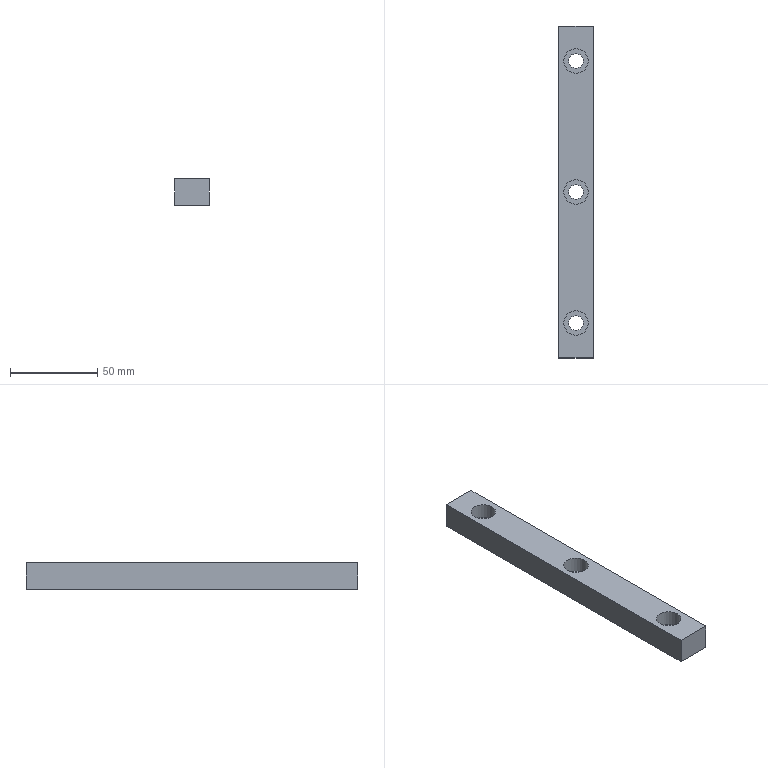Part | STEP file | YBQDJ-QD-4 | 1 solid | 15 faces | box 20 x 190 x 15 mm | volume 51822 mm3 | plane 9 | cylinder 6 | commonest cylinder face diameters 8.5 x3 14 x3
STEP:
#1=CARTESIAN_POINT('',(0.,0.,0.));
#2=DIRECTION('',(0.,0.,1.));
#3=DIRECTION('',(1.,0.,0.));
#4=AXIS2_PLACEMENT_3D('',#1,#2,#3);
#5=CARTESIAN_POINT('',(-330.,-100.,120.));
#6=VERTEX_POINT('',#5);
#7=CARTESIAN_POINT('',(-330.,-290.,120.));
#8=VERTEX_POINT('',#7);
#9=CARTESIAN_POINT('',(-330.,-85.,120.));
#10=DIRECTION('',(0.,-1.,0.));
#11=VECTOR('',#10,1.);
#12=LINE('',#9,#11);
#13=CARTESIAN_POINT('',(-330.,-85.,135.));
#14=DIRECTION('',(1.,0.,0.));
#15=DIRECTION('',(0.,0.,-1.));
#16=AXIS2_PLACEMENT_3D('',#13,#14,#15);
#17=PLANE('',#16);
#18=CARTESIAN_POINT('',(15.,0.));
#19=DIRECTION('',(0.,-1.));
#20=VECTOR('',#19,1.);
#21=LINE('',#18,#20);
#22=(GEOMETRIC_REPRESENTATION_CONTEXT(2)PARAMETRIC_REPRESENTATION_CONTEXT()REPRESENTATION_CONTEXT('',''));
#23=DEFINITIONAL_REPRESENTATION('',(#21),#22);
#24=PCURVE('',#17,#23);
#25=CARTESIAN_POINT('',(92.5,0.000000001,120.));
#26=DIRECTION('',(0.,0.,1.));
#27=DIRECTION('',(1.,0.,0.));
#28=AXIS2_PLACEMENT_3D('',#25,#26,#27);
#29=PLANE('',#28);
#30=CARTESIAN_POINT('',(-422.5,-85.));
#31=DIRECTION('',(0.,-1.));
#32=VECTOR('',#31,1.);
#33=LINE('',#30,#32);
#34=(GEOMETRIC_REPRESENTATION_CONTEXT(2)PARAMETRIC_REPRESENTATION_CONTEXT()REPRESENTATION_CONTEXT('',''));
#35=DEFINITIONAL_REPRESENTATION('',(#33),#34);
#36=PCURVE('',#29,#35);
#37=SURFACE_CURVE('',#12,(#24,#36),.PCURVE_S1.);
#38=EDGE_CURVE('',#6,#8,#37,.T.);
#39=ORIENTED_EDGE('',*,*,#38,.T.);
#40=CARTESIAN_POINT('',(-330.,-290.,135.));
#41=VERTEX_POINT('',#40);
#42=CARTESIAN_POINT('',(-330.,-290.,9.));
#43=DIRECTION('',(0.,0.,-1.));
#44=VECTOR('',#43,1.);
#45=LINE('',#42,#44);
#46=CARTESIAN_POINT('',(126.,-205.));
#47=DIRECTION('',(1.,0.));
#48=VECTOR('',#47,1.);
#49=LINE('',#46,#48);
#50=(GEOMETRIC_REPRESENTATION_CONTEXT(2)PARAMETRIC_REPRESENTATION_CONTEXT()REPRESENTATION_CONTEXT('',''));
#51=DEFINITIONAL_REPRESENTATION('',(#49),#50);
#52=PCURVE('',#17,#51);
#53=CARTESIAN_POINT('',(163.5,-290.,9.));
#54=DIRECTION('',(0.,-1.,0.));
#55=DIRECTION('',(0.,0.,-1.));
#56=AXIS2_PLACEMENT_3D('',#53,#54,#55);
#57=PLANE('',#56);
#58=CARTESIAN_POINT('',(0.,-493.5));
#59=DIRECTION('',(1.,0.));
#60=VECTOR('',#59,1.);
#61=LINE('',#58,#60);
#62=(GEOMETRIC_REPRESENTATION_CONTEXT(2)PARAMETRIC_REPRESENTATION_CONTEXT()REPRESENTATION_CONTEXT('',''));
#63=DEFINITIONAL_REPRESENTATION('',(#61),#62);
#64=PCURVE('',#57,#63);
#65=SURFACE_CURVE('',#45,(#52,#64),.PCURVE_S1.);
#66=EDGE_CURVE('',#41,#8,#65,.T.);
#67=ORIENTED_EDGE('',*,*,#66,.F.);
#68=CARTESIAN_POINT('',(-330.,-100.,135.));
#69=VERTEX_POINT('',#68);
#70=CARTESIAN_POINT('',(-330.,-85.,135.));
#71=DIRECTION('',(0.,-1.,0.));
#72=VECTOR('',#71,1.);
#73=LINE('',#70,#72);
#74=CARTESIAN_POINT('',(0.,0.));
#75=DIRECTION('',(0.,-1.));
#76=VECTOR('',#75,1.);
#77=LINE('',#74,#76);
#78=(GEOMETRIC_REPRESENTATION_CONTEXT(2)PARAMETRIC_REPRESENTATION_CONTEXT()REPRESENTATION_CONTEXT('',''));
#79=DEFINITIONAL_REPRESENTATION('',(#77),#78);
#80=PCURVE('',#17,#79);
#81=CARTESIAN_POINT('',(-341.,1779.,135.));
#82=DIRECTION('',(0.,0.,1.));
#83=DIRECTION('',(1.,0.,0.));
#84=AXIS2_PLACEMENT_3D('',#81,#82,#83);
#85=PLANE('',#84);
#86=CARTESIAN_POINT('',(11.,-1864.));
#87=DIRECTION('',(0.,-1.));
#88=VECTOR('',#87,1.);
#89=LINE('',#86,#88);
#90=(GEOMETRIC_REPRESENTATION_CONTEXT(2)PARAMETRIC_REPRESENTATION_CONTEXT()REPRESENTATION_CONTEXT('',''));
#91=DEFINITIONAL_REPRESENTATION('',(#89),#90);
#92=PCURVE('',#85,#91);
#93=SURFACE_CURVE('',#73,(#80,#92),.PCURVE_S1.);
#94=EDGE_CURVE('',#69,#41,#93,.T.);
#95=ORIENTED_EDGE('',*,*,#94,.F.);
#96=CARTESIAN_POINT('',(-330.,-100.,135.));
#97=DIRECTION('',(0.,0.,-1.));
#98=VECTOR('',#97,1.);
#99=LINE('',#96,#98);
#100=CARTESIAN_POINT('',(0.,-15.));
#101=DIRECTION('',(1.,0.));
#102=VECTOR('',#101,1.);
#103=LINE('',#100,#102);
#104=(GEOMETRIC_REPRESENTATION_CONTEXT(2)PARAMETRIC_REPRESENTATION_CONTEXT()REPRESENTATION_CONTEXT('',''));
#105=DEFINITIONAL_REPRESENTATION('',(#103),#104);
#106=PCURVE('',#17,#105);
#107=CARTESIAN_POINT('',(-292.,-100.,264.));
#108=DIRECTION('',(0.,-1.,0.));
#109=DIRECTION('',(0.,0.,1.));
#110=AXIS2_PLACEMENT_3D('',#107,#108,#109);
#111=PLANE('',#110);
#112=CARTESIAN_POINT('',(-129.,38.));
#113=DIRECTION('',(-1.,0.));
#114=VECTOR('',#113,1.);
#115=LINE('',#112,#114);
#116=(GEOMETRIC_REPRESENTATION_CONTEXT(2)PARAMETRIC_REPRESENTATION_CONTEXT()REPRESENTATION_CONTEXT('',''));
#117=DEFINITIONAL_REPRESENTATION('',(#115),#116);
#118=PCURVE('',#111,#117);
#119=SURFACE_CURVE('',#99,(#106,#118),.PCURVE_S1.);
#120=EDGE_CURVE('',#69,#6,#119,.T.);
#121=ORIENTED_EDGE('',*,*,#120,.T.);
#122=EDGE_LOOP('',(#39,#67,#95,#121));
#123=FACE_BOUND('',#122,.T.);
#124=ADVANCED_FACE('',(#123),#17,.F.);
#125=CARTESIAN_POINT('',(-310.,-290.,120.));
#126=VERTEX_POINT('',#125);
#127=CARTESIAN_POINT('',(163.5,-290.,120.));
#128=DIRECTION('',(1.,0.,0.));
#129=VECTOR('',#128,1.);
#130=LINE('',#127,#129);
#131=CARTESIAN_POINT('',(-111.,0.));
#132=DIRECTION('',(0.,1.));
#133=VECTOR('',#132,1.);
#134=LINE('',#131,#133);
#135=(GEOMETRIC_REPRESENTATION_CONTEXT(2)PARAMETRIC_REPRESENTATION_CONTEXT()REPRESENTATION_CONTEXT('',''));
#136=DEFINITIONAL_REPRESENTATION('',(#134),#135);
#137=PCURVE('',#57,#136);
#138=CARTESIAN_POINT('',(71.,-290.));
#139=DIRECTION('',(1.,0.));
#140=VECTOR('',#139,1.);
#141=LINE('',#138,#140);
#142=(GEOMETRIC_REPRESENTATION_CONTEXT(2)PARAMETRIC_REPRESENTATION_CONTEXT()REPRESENTATION_CONTEXT('',''));
#143=DEFINITIONAL_REPRESENTATION('',(#141),#142);
#144=PCURVE('',#29,#143);
#145=SURFACE_CURVE('',#130,(#137,#144),.PCURVE_S1.);
#146=EDGE_CURVE('',#8,#126,#145,.T.);
#147=ORIENTED_EDGE('',*,*,#146,.T.);
#148=CARTESIAN_POINT('',(-310.,-290.,135.));
#149=VERTEX_POINT('',#148);
#150=CARTESIAN_POINT('',(-310.,-290.,135.));
#151=DIRECTION('',(0.,0.,-1.));
#152=VECTOR('',#151,1.);
#153=LINE('',#150,#152);
#154=CARTESIAN_POINT('',(-126.,-473.5));
#155=DIRECTION('',(1.,0.));
#156=VECTOR('',#155,1.);
#157=LINE('',#154,#156);
#158=(GEOMETRIC_REPRESENTATION_CONTEXT(2)PARAMETRIC_REPRESENTATION_CONTEXT()REPRESENTATION_CONTEXT('',''));
#159=DEFINITIONAL_REPRESENTATION('',(#157),#158);
#160=PCURVE('',#57,#159);
#161=CARTESIAN_POINT('',(-310.,-305.,135.));
#162=DIRECTION('',(-1.,0.,0.));
#163=DIRECTION('',(0.,0.,1.));
#164=AXIS2_PLACEMENT_3D('',#161,#162,#163);
#165=PLANE('',#164);
#166=CARTESIAN_POINT('',(0.,15.));
#167=DIRECTION('',(-1.,0.));
#168=VECTOR('',#167,1.);
#169=LINE('',#166,#168);
#170=(GEOMETRIC_REPRESENTATION_CONTEXT(2)PARAMETRIC_REPRESENTATION_CONTEXT()REPRESENTATION_CONTEXT('',''));
#171=DEFINITIONAL_REPRESENTATION('',(#169),#170);
#172=PCURVE('',#165,#171);
#173=SURFACE_CURVE('',#153,(#160,#172),.PCURVE_S1.);
#174=EDGE_CURVE('',#149,#126,#173,.T.);
#175=ORIENTED_EDGE('',*,*,#174,.F.);
#176=CARTESIAN_POINT('',(163.5,-290.,135.));
#177=DIRECTION('',(1.,0.,0.));
#178=VECTOR('',#177,1.);
#179=LINE('',#176,#178);
#180=CARTESIAN_POINT('',(-126.,0.));
#181=DIRECTION('',(0.,1.));
#182=VECTOR('',#181,1.);
#183=LINE('',#180,#182);
#184=(GEOMETRIC_REPRESENTATION_CONTEXT(2)PARAMETRIC_REPRESENTATION_CONTEXT()REPRESENTATION_CONTEXT('',''));
#185=DEFINITIONAL_REPRESENTATION('',(#183),#184);
#186=PCURVE('',#57,#185);
#187=CARTESIAN_POINT('',(504.5,-2069.));
#188=DIRECTION('',(1.,0.));
#189=VECTOR('',#188,1.);
#190=LINE('',#187,#189);
#191=(GEOMETRIC_REPRESENTATION_CONTEXT(2)PARAMETRIC_REPRESENTATION_CONTEXT()REPRESENTATION_CONTEXT('',''));
#192=DEFINITIONAL_REPRESENTATION('',(#190),#191);
#193=PCURVE('',#85,#192);
#194=SURFACE_CURVE('',#179,(#186,#193),.PCURVE_S1.);
#195=EDGE_CURVE('',#41,#149,#194,.T.);
#196=ORIENTED_EDGE('',*,*,#195,.F.);
#197=ORIENTED_EDGE('',*,*,#66,.T.);
#198=EDGE_LOOP('',(#147,#175,#196,#197));
#199=FACE_BOUND('',#198,.T.);
#200=ADVANCED_FACE('',(#199),#57,.T.);
#201=CARTESIAN_POINT('',(-310.,-100.,120.));
#202=VERTEX_POINT('',#201);
#203=CARTESIAN_POINT('',(-310.,-305.,120.));
#204=DIRECTION('',(0.,1.,0.));
#205=VECTOR('',#204,1.);
#206=LINE('',#203,#205);
#207=CARTESIAN_POINT('',(-15.,0.));
#208=DIRECTION('',(0.,1.));
#209=VECTOR('',#208,1.);
#210=LINE('',#207,#209);
#211=(GEOMETRIC_REPRESENTATION_CONTEXT(2)PARAMETRIC_REPRESENTATION_CONTEXT()REPRESENTATION_CONTEXT('',''));
#212=DEFINITIONAL_REPRESENTATION('',(#210),#211);
#213=PCURVE('',#165,#212);
#214=CARTESIAN_POINT('',(-402.5,-305.));
#215=DIRECTION('',(0.,1.));
#216=VECTOR('',#215,1.);
#217=LINE('',#214,#216);
#218=(GEOMETRIC_REPRESENTATION_CONTEXT(2)PARAMETRIC_REPRESENTATION_CONTEXT()REPRESENTATION_CONTEXT('',''));
#219=DEFINITIONAL_REPRESENTATION('',(#217),#218);
#220=PCURVE('',#29,#219);
#221=SURFACE_CURVE('',#206,(#213,#220),.PCURVE_S1.);
#222=EDGE_CURVE('',#126,#202,#221,.T.);
#223=ORIENTED_EDGE('',*,*,#222,.T.);
#224=CARTESIAN_POINT('',(-310.,-100.,135.));
#225=VERTEX_POINT('',#224);
#226=CARTESIAN_POINT('',(-310.,-100.,264.));
#227=DIRECTION('',(0.,0.,-1.));
#228=VECTOR('',#227,1.);
#229=LINE('',#226,#228);
#230=CARTESIAN_POINT('',(129.,205.));
#231=DIRECTION('',(-1.,0.));
#232=VECTOR('',#231,1.);
#233=LINE('',#230,#232);
#234=(GEOMETRIC_REPRESENTATION_CONTEXT(2)PARAMETRIC_REPRESENTATION_CONTEXT()REPRESENTATION_CONTEXT('',''));
#235=DEFINITIONAL_REPRESENTATION('',(#233),#234);
#236=PCURVE('',#165,#235);
#237=CARTESIAN_POINT('',(0.,18.));
#238=DIRECTION('',(-1.,0.));
#239=VECTOR('',#238,1.);
#240=LINE('',#237,#239);
#241=(GEOMETRIC_REPRESENTATION_CONTEXT(2)PARAMETRIC_REPRESENTATION_CONTEXT()REPRESENTATION_CONTEXT('',''));
#242=DEFINITIONAL_REPRESENTATION('',(#240),#241);
#243=PCURVE('',#111,#242);
#244=SURFACE_CURVE('',#229,(#236,#243),.PCURVE_S1.);
#245=EDGE_CURVE('',#225,#202,#244,.T.);
#246=ORIENTED_EDGE('',*,*,#245,.F.);
#247=CARTESIAN_POINT('',(-310.,-305.,135.));
#248=DIRECTION('',(0.,1.,0.));
#249=VECTOR('',#248,1.);
#250=LINE('',#247,#249);
#251=CARTESIAN_POINT('',(0.,0.));
#252=DIRECTION('',(0.,1.));
#253=VECTOR('',#252,1.);
#254=LINE('',#251,#253);
#255=(GEOMETRIC_REPRESENTATION_CONTEXT(2)PARAMETRIC_REPRESENTATION_CONTEXT()REPRESENTATION_CONTEXT('',''));
#256=DEFINITIONAL_REPRESENTATION('',(#254),#255);
#257=PCURVE('',#165,#256);
#258=CARTESIAN_POINT('',(31.,-2084.));
#259=DIRECTION('',(0.,1.));
#260=VECTOR('',#259,1.);
#261=LINE('',#258,#260);
#262=(GEOMETRIC_REPRESENTATION_CONTEXT(2)PARAMETRIC_REPRESENTATION_CONTEXT()REPRESENTATION_CONTEXT('',''));
#263=DEFINITIONAL_REPRESENTATION('',(#261),#262);
#264=PCURVE('',#85,#263);
#265=SURFACE_CURVE('',#250,(#257,#264),.PCURVE_S1.);
#266=EDGE_CURVE('',#149,#225,#265,.T.);
#267=ORIENTED_EDGE('',*,*,#266,.F.);
#268=ORIENTED_EDGE('',*,*,#174,.T.);
#269=EDGE_LOOP('',(#223,#246,#267,#268));
#270=FACE_BOUND('',#269,.T.);
#271=ADVANCED_FACE('',(#270),#165,.F.);
#272=CARTESIAN_POINT('',(-292.,-100.,120.));
#273=DIRECTION('',(-1.,0.,0.));
#274=VECTOR('',#273,1.);
#275=LINE('',#272,#274);
#276=CARTESIAN_POINT('',(-144.,0.));
#277=DIRECTION('',(0.,1.));
#278=VECTOR('',#277,1.);
#279=LINE('',#276,#278);
#280=(GEOMETRIC_REPRESENTATION_CONTEXT(2)PARAMETRIC_REPRESENTATION_CONTEXT()REPRESENTATION_CONTEXT('',''));
#281=DEFINITIONAL_REPRESENTATION('',(#279),#280);
#282=PCURVE('',#111,#281);
#283=CARTESIAN_POINT('',(-384.5,-100.));
#284=DIRECTION('',(-1.,0.));
#285=VECTOR('',#284,1.);
#286=LINE('',#283,#285);
#287=(GEOMETRIC_REPRESENTATION_CONTEXT(2)PARAMETRIC_REPRESENTATION_CONTEXT()REPRESENTATION_CONTEXT('',''));
#288=DEFINITIONAL_REPRESENTATION('',(#286),#287);
#289=PCURVE('',#29,#288);
#290=SURFACE_CURVE('',#275,(#282,#289),.PCURVE_S1.);
#291=EDGE_CURVE('',#202,#6,#290,.T.);
#292=ORIENTED_EDGE('',*,*,#291,.T.);
#293=ORIENTED_EDGE('',*,*,#120,.F.);
#294=CARTESIAN_POINT('',(-292.,-100.,135.));
#295=DIRECTION('',(-1.,0.,0.));
#296=VECTOR('',#295,1.);
#297=LINE('',#294,#296);
#298=CARTESIAN_POINT('',(-129.,0.));
#299=DIRECTION('',(0.,1.));
#300=VECTOR('',#299,1.);
#301=LINE('',#298,#300);
#302=(GEOMETRIC_REPRESENTATION_CONTEXT(2)PARAMETRIC_REPRESENTATION_CONTEXT()REPRESENTATION_CONTEXT('',''));
#303=DEFINITIONAL_REPRESENTATION('',(#301),#302);
#304=PCURVE('',#111,#303);
#305=CARTESIAN_POINT('',(49.,-1879.));
#306=DIRECTION('',(-1.,0.));
#307=VECTOR('',#306,1.);
#308=LINE('',#305,#307);
#309=(GEOMETRIC_REPRESENTATION_CONTEXT(2)PARAMETRIC_REPRESENTATION_CONTEXT()REPRESENTATION_CONTEXT('',''));
#310=DEFINITIONAL_REPRESENTATION('',(#308),#309);
#311=PCURVE('',#85,#310);
#312=SURFACE_CURVE('',#297,(#304,#311),.PCURVE_S1.);
#313=EDGE_CURVE('',#225,#69,#312,.T.);
#314=ORIENTED_EDGE('',*,*,#313,.F.);
#315=ORIENTED_EDGE('',*,*,#245,.T.);
#316=EDGE_LOOP('',(#292,#293,#314,#315));
#317=FACE_BOUND('',#316,.T.);
#318=ADVANCED_FACE('',(#317),#111,.F.);
#319=CARTESIAN_POINT('',(-313.,-270.,135.));
#320=VERTEX_POINT('',#319);
#321=CARTESIAN_POINT('',(-327.,-270.,135.));
#322=VERTEX_POINT('',#321);
#323=CARTESIAN_POINT('',(-320.,-270.,135.));
#324=DIRECTION('',(0.,0.,-1.));
#325=DIRECTION('',(1.,0.,0.));
#326=AXIS2_PLACEMENT_3D('',#323,#324,#325);
#327=CIRCLE('',#326,7.);
#328=CARTESIAN_POINT('',(28.,-2049.));
#329=CARTESIAN_POINT('',(28.,-2061.124));
#330=CARTESIAN_POINT('',(17.5,-2055.062));
#331=CARTESIAN_POINT('',(7.,-2049.));
#332=CARTESIAN_POINT('',(17.5,-2042.938));
#333=CARTESIAN_POINT('',(28.,-2036.876));
#334=CARTESIAN_POINT('',(28.,-2049.));
#335=(BOUNDED_CURVE()B_SPLINE_CURVE(2,(#328,#329,#330,#331,#332,#333,#334),.UNSPECIFIED.,.T.,.F.)B_SPLINE_CURVE_WITH_KNOTS((1,2,2,2,2,1),(-2.094,0.,2.094,4.189,6.283,8.378),.UNSPECIFIED.)CURVE()GEOMETRIC_REPRESENTATION_ITEM()RATIONAL_B_SPLINE_CURVE((1.,0.5,1.,0.5,1.,0.5,1.))REPRESENTATION_ITEM(''));
#336=(GEOMETRIC_REPRESENTATION_CONTEXT(2)PARAMETRIC_REPRESENTATION_CONTEXT()REPRESENTATION_CONTEXT('',''));
#337=DEFINITIONAL_REPRESENTATION('',(#335),#336);
#338=PCURVE('',#85,#337);
#339=CARTESIAN_POINT('',(-320.,-270.,133.));
#340=DIRECTION('',(0.,0.,-1.));
#341=DIRECTION('',(-1.,0.,0.));
#342=AXIS2_PLACEMENT_3D('',#339,#340,#341);
#343=CYLINDRICAL_SURFACE('',#342,7.);
#344=CARTESIAN_POINT('',(3.142,-2.));
#345=DIRECTION('',(1.,0.));
#346=VECTOR('',#345,1.);
#347=LINE('',#344,#346);
#348=(GEOMETRIC_REPRESENTATION_CONTEXT(2)PARAMETRIC_REPRESENTATION_CONTEXT()REPRESENTATION_CONTEXT('',''));
#349=DEFINITIONAL_REPRESENTATION('',(#347),#348);
#350=PCURVE('',#343,#349);
#351=SURFACE_CURVE('',#327,(#338,#350),.PCURVE_S1.);
#352=EDGE_CURVE('',#320,#322,#351,.T.);
#353=ORIENTED_EDGE('',*,*,#352,.T.);
#354=CARTESIAN_POINT('',(-320.,-270.,135.));
#355=DIRECTION('',(0.,0.,-1.));
#356=DIRECTION('',(1.,0.,0.));
#357=AXIS2_PLACEMENT_3D('',#354,#355,#356);
#358=CIRCLE('',#357,7.);
#359=CARTESIAN_POINT('',(28.,-2049.));
#360=CARTESIAN_POINT('',(28.,-2061.124));
#361=CARTESIAN_POINT('',(17.5,-2055.062));
#362=CARTESIAN_POINT('',(7.,-2049.));
#363=CARTESIAN_POINT('',(17.5,-2042.938));
#364=CARTESIAN_POINT('',(28.,-2036.876));
#365=CARTESIAN_POINT('',(28.,-2049.));
#366=(BOUNDED_CURVE()B_SPLINE_CURVE(2,(#359,#360,#361,#362,#363,#364,#365),.UNSPECIFIED.,.T.,.F.)B_SPLINE_CURVE_WITH_KNOTS((1,2,2,2,2,1),(-2.094,0.,2.094,4.189,6.283,8.378),.UNSPECIFIED.)CURVE()GEOMETRIC_REPRESENTATION_ITEM()RATIONAL_B_SPLINE_CURVE((1.,0.5,1.,0.5,1.,0.5,1.))REPRESENTATION_ITEM(''));
#367=(GEOMETRIC_REPRESENTATION_CONTEXT(2)PARAMETRIC_REPRESENTATION_CONTEXT()REPRESENTATION_CONTEXT('',''));
#368=DEFINITIONAL_REPRESENTATION('',(#366),#367);
#369=PCURVE('',#85,#368);
#370=CARTESIAN_POINT('',(-3.142,-2.));
#371=DIRECTION('',(1.,0.));
#372=VECTOR('',#371,1.);
#373=LINE('',#370,#372);
#374=(GEOMETRIC_REPRESENTATION_CONTEXT(2)PARAMETRIC_REPRESENTATION_CONTEXT()REPRESENTATION_CONTEXT('',''));
#375=DEFINITIONAL_REPRESENTATION('',(#373),#374);
#376=PCURVE('',#343,#375);
#377=SURFACE_CURVE('',#358,(#369,#376),.PCURVE_S1.);
#378=EDGE_CURVE('',#322,#320,#377,.T.);
#379=ORIENTED_EDGE('',*,*,#378,.T.);
#380=EDGE_LOOP('',(#353,#379));
#381=FACE_BOUND('',#380,.T.);
#382=CARTESIAN_POINT('',(-313.,-195.,135.));
#383=VERTEX_POINT('',#382);
#384=CARTESIAN_POINT('',(-327.,-195.,135.));
#385=VERTEX_POINT('',#384);
#386=CARTESIAN_POINT('',(-320.,-195.,135.));
#387=DIRECTION('',(0.,0.,-1.));
#388=DIRECTION('',(1.,0.,0.));
#389=AXIS2_PLACEMENT_3D('',#386,#387,#388);
#390=CIRCLE('',#389,7.);
#391=CARTESIAN_POINT('',(28.,-1974.));
#392=CARTESIAN_POINT('',(28.,-1986.124));
#393=CARTESIAN_POINT('',(17.5,-1980.062));
#394=CARTESIAN_POINT('',(7.,-1974.));
#395=CARTESIAN_POINT('',(17.5,-1967.938));
#396=CARTESIAN_POINT('',(28.,-1961.876));
#397=CARTESIAN_POINT('',(28.,-1974.));
#398=(BOUNDED_CURVE()B_SPLINE_CURVE(2,(#391,#392,#393,#394,#395,#396,#397),.UNSPECIFIED.,.T.,.F.)B_SPLINE_CURVE_WITH_KNOTS((1,2,2,2,2,1),(-2.094,0.,2.094,4.189,6.283,8.378),.UNSPECIFIED.)CURVE()GEOMETRIC_REPRESENTATION_ITEM()RATIONAL_B_SPLINE_CURVE((1.,0.5,1.,0.5,1.,0.5,1.))REPRESENTATION_ITEM(''));
#399=(GEOMETRIC_REPRESENTATION_CONTEXT(2)PARAMETRIC_REPRESENTATION_CONTEXT()REPRESENTATION_CONTEXT('',''));
#400=DEFINITIONAL_REPRESENTATION('',(#398),#399);
#401=PCURVE('',#85,#400);
#402=CARTESIAN_POINT('',(-320.,-195.,133.));
#403=DIRECTION('',(0.,0.,-1.));
#404=DIRECTION('',(-1.,0.,0.));
#405=AXIS2_PLACEMENT_3D('',#402,#403,#404);
#406=CYLINDRICAL_SURFACE('',#405,7.);
#407=CARTESIAN_POINT('',(3.142,-2.));
#408=DIRECTION('',(1.,0.));
#409=VECTOR('',#408,1.);
#410=LINE('',#407,#409);
#411=(GEOMETRIC_REPRESENTATION_CONTEXT(2)PARAMETRIC_REPRESENTATION_CONTEXT()REPRESENTATION_CONTEXT('',''));
#412=DEFINITIONAL_REPRESENTATION('',(#410),#411);
#413=PCURVE('',#406,#412);
#414=SURFACE_CURVE('',#390,(#401,#413),.PCURVE_S1.);
#415=EDGE_CURVE('',#383,#385,#414,.T.);
#416=ORIENTED_EDGE('',*,*,#415,.T.);
#417=CARTESIAN_POINT('',(-320.,-195.,135.));
#418=DIRECTION('',(0.,0.,-1.));
#419=DIRECTION('',(1.,0.,0.));
#420=AXIS2_PLACEMENT_3D('',#417,#418,#419);
#421=CIRCLE('',#420,7.);
#422=CARTESIAN_POINT('',(28.,-1974.));
#423=CARTESIAN_POINT('',(28.,-1986.124));
#424=CARTESIAN_POINT('',(17.5,-1980.062));
#425=CARTESIAN_POINT('',(7.,-1974.));
#426=CARTESIAN_POINT('',(17.5,-1967.938));
#427=CARTESIAN_POINT('',(28.,-1961.876));
#428=CARTESIAN_POINT('',(28.,-1974.));
#429=(BOUNDED_CURVE()B_SPLINE_CURVE(2,(#422,#423,#424,#425,#426,#427,#428),.UNSPECIFIED.,.T.,.F.)B_SPLINE_CURVE_WITH_KNOTS((1,2,2,2,2,1),(-2.094,0.,2.094,4.189,6.283,8.378),.UNSPECIFIED.)CURVE()GEOMETRIC_REPRESENTATION_ITEM()RATIONAL_B_SPLINE_CURVE((1.,0.5,1.,0.5,1.,0.5,1.))REPRESENTATION_ITEM(''));
#430=(GEOMETRIC_REPRESENTATION_CONTEXT(2)PARAMETRIC_REPRESENTATION_CONTEXT()REPRESENTATION_CONTEXT('',''));
#431=DEFINITIONAL_REPRESENTATION('',(#429),#430);
#432=PCURVE('',#85,#431);
#433=CARTESIAN_POINT('',(-3.142,-2.));
#434=DIRECTION('',(1.,0.));
#435=VECTOR('',#434,1.);
#436=LINE('',#433,#435);
#437=(GEOMETRIC_REPRESENTATION_CONTEXT(2)PARAMETRIC_REPRESENTATION_CONTEXT()REPRESENTATION_CONTEXT('',''));
#438=DEFINITIONAL_REPRESENTATION('',(#436),#437);
#439=PCURVE('',#406,#438);
#440=SURFACE_CURVE('',#421,(#432,#439),.PCURVE_S1.);
#441=EDGE_CURVE('',#385,#383,#440,.T.);
#442=ORIENTED_EDGE('',*,*,#441,.T.);
#443=EDGE_LOOP('',(#416,#442));
#444=FACE_BOUND('',#443,.T.);
#445=CARTESIAN_POINT('',(-313.,-120.,135.));
#446=VERTEX_POINT('',#445);
#447=CARTESIAN_POINT('',(-327.,-120.,135.));
#448=VERTEX_POINT('',#447);
#449=CARTESIAN_POINT('',(-320.,-120.,135.));
#450=DIRECTION('',(0.,0.,-1.));
#451=DIRECTION('',(1.,0.,0.));
#452=AXIS2_PLACEMENT_3D('',#449,#450,#451);
#453=CIRCLE('',#452,7.);
#454=CARTESIAN_POINT('',(28.,-1899.));
#455=CARTESIAN_POINT('',(28.,-1911.124));
#456=CARTESIAN_POINT('',(17.5,-1905.062));
#457=CARTESIAN_POINT('',(7.,-1899.));
#458=CARTESIAN_POINT('',(17.5,-1892.938));
#459=CARTESIAN_POINT('',(28.,-1886.876));
#460=CARTESIAN_POINT('',(28.,-1899.));
#461=(BOUNDED_CURVE()B_SPLINE_CURVE(2,(#454,#455,#456,#457,#458,#459,#460),.UNSPECIFIED.,.T.,.F.)B_SPLINE_CURVE_WITH_KNOTS((1,2,2,2,2,1),(-2.094,0.,2.094,4.189,6.283,8.378),.UNSPECIFIED.)CURVE()GEOMETRIC_REPRESENTATION_ITEM()RATIONAL_B_SPLINE_CURVE((1.,0.5,1.,0.5,1.,0.5,1.))REPRESENTATION_ITEM(''));
#462=(GEOMETRIC_REPRESENTATION_CONTEXT(2)PARAMETRIC_REPRESENTATION_CONTEXT()REPRESENTATION_CONTEXT('',''));
#463=DEFINITIONAL_REPRESENTATION('',(#461),#462);
#464=PCURVE('',#85,#463);
#465=CARTESIAN_POINT('',(-320.,-120.,133.));
#466=DIRECTION('',(0.,0.,-1.));
#467=DIRECTION('',(-1.,0.,0.));
#468=AXIS2_PLACEMENT_3D('',#465,#466,#467);
#469=CYLINDRICAL_SURFACE('',#468,7.);
#470=CARTESIAN_POINT('',(3.142,-2.));
#471=DIRECTION('',(1.,0.));
#472=VECTOR('',#471,1.);
#473=LINE('',#470,#472);
#474=(GEOMETRIC_REPRESENTATION_CONTEXT(2)PARAMETRIC_REPRESENTATION_CONTEXT()REPRESENTATION_CONTEXT('',''));
#475=DEFINITIONAL_REPRESENTATION('',(#473),#474);
#476=PCURVE('',#469,#475);
#477=SURFACE_CURVE('',#453,(#464,#476),.PCURVE_S1.);
#478=EDGE_CURVE('',#446,#448,#477,.T.);
#479=ORIENTED_EDGE('',*,*,#478,.T.);
#480=CARTESIAN_POINT('',(-320.,-120.,135.));
#481=DIRECTION('',(0.,0.,-1.));
#482=DIRECTION('',(1.,0.,0.));
#483=AXIS2_PLACEMENT_3D('',#480,#481,#482);
#484=CIRCLE('',#483,7.);
#485=CARTESIAN_POINT('',(28.,-1899.));
#486=CARTESIAN_POINT('',(28.,-1911.124));
#487=CARTESIAN_POINT('',(17.5,-1905.062));
#488=CARTESIAN_POINT('',(7.,-1899.));
#489=CARTESIAN_POINT('',(17.5,-1892.938));
#490=CARTESIAN_POINT('',(28.,-1886.876));
#491=CARTESIAN_POINT('',(28.,-1899.));
#492=(BOUNDED_CURVE()B_SPLINE_CURVE(2,(#485,#486,#487,#488,#489,#490,#491),.UNSPECIFIED.,.T.,.F.)B_SPLINE_CURVE_WITH_KNOTS((1,2,2,2,2,1),(-2.094,0.,2.094,4.189,6.283,8.378),.UNSPECIFIED.)CURVE()GEOMETRIC_REPRESENTATION_ITEM()RATIONAL_B_SPLINE_CURVE((1.,0.5,1.,0.5,1.,0.5,1.))REPRESENTATION_ITEM(''));
#493=(GEOMETRIC_REPRESENTATION_CONTEXT(2)PARAMETRIC_REPRESENTATION_CONTEXT()REPRESENTATION_CONTEXT('',''));
#494=DEFINITIONAL_REPRESENTATION('',(#492),#493);
#495=PCURVE('',#85,#494);
#496=CARTESIAN_POINT('',(-3.142,-2.));
#497=DIRECTION('',(1.,0.));
#498=VECTOR('',#497,1.);
#499=LINE('',#496,#498);
#500=(GEOMETRIC_REPRESENTATION_CONTEXT(2)PARAMETRIC_REPRESENTATION_CONTEXT()REPRESENTATION_CONTEXT('',''));
#501=DEFINITIONAL_REPRESENTATION('',(#499),#500);
#502=PCURVE('',#469,#501);
#503=SURFACE_CURVE('',#484,(#495,#502),.PCURVE_S1.);
#504=EDGE_CURVE('',#448,#446,#503,.T.);
#505=ORIENTED_EDGE('',*,*,#504,.T.);
#506=EDGE_LOOP('',(#479,#505));
#507=FACE_BOUND('',#506,.T.);
#508=ORIENTED_EDGE('',*,*,#94,.T.);
#509=ORIENTED_EDGE('',*,*,#195,.T.);
#510=ORIENTED_EDGE('',*,*,#266,.T.);
#511=ORIENTED_EDGE('',*,*,#313,.T.);
#512=EDGE_LOOP('',(#508,#509,#510,#511));
#513=FACE_BOUND('',#512,.T.);
#514=ADVANCED_FACE('',(#381,#444,#507,#513),#85,.T.);
#515=CARTESIAN_POINT('',(-315.75,-270.,120.));
#516=VERTEX_POINT('',#515);
#517=CARTESIAN_POINT('',(-324.25,-270.,120.));
#518=VERTEX_POINT('',#517);
#519=CARTESIAN_POINT('',(-320.,-270.,120.));
#520=DIRECTION('',(0.,0.,1.));
#521=DIRECTION('',(1.,0.,0.));
#522=AXIS2_PLACEMENT_3D('',#519,#520,#521);
#523=CIRCLE('',#522,4.25);
#524=CARTESIAN_POINT('',(-412.5,-270.));
#525=DIRECTION('',(1.,0.));
#526=AXIS2_PLACEMENT_2D('',#524,#525);
#527=CIRCLE('',#526,4.25);
#528=(GEOMETRIC_REPRESENTATION_CONTEXT(2)PARAMETRIC_REPRESENTATION_CONTEXT()REPRESENTATION_CONTEXT('',''));
#529=DEFINITIONAL_REPRESENTATION('',(#527),#528);
#530=PCURVE('',#29,#529);
#531=CARTESIAN_POINT('',(-320.,-270.,52.558));
#532=DIRECTION('',(0.,0.,-1.));
#533=DIRECTION('',(-1.,0.,0.));
#534=AXIS2_PLACEMENT_3D('',#531,#532,#533);
#535=CYLINDRICAL_SURFACE('',#534,4.25);
#536=CARTESIAN_POINT('',(3.142,-67.442));
#537=DIRECTION('',(-1.,0.));
#538=VECTOR('',#537,1.);
#539=LINE('',#536,#538);
#540=(GEOMETRIC_REPRESENTATION_CONTEXT(2)PARAMETRIC_REPRESENTATION_CONTEXT()REPRESENTATION_CONTEXT('',''));
#541=DEFINITIONAL_REPRESENTATION('',(#539),#540);
#542=PCURVE('',#535,#541);
#543=SURFACE_CURVE('',#523,(#530,#542),.PCURVE_S1.);
#544=EDGE_CURVE('',#516,#518,#543,.T.);
#545=ORIENTED_EDGE('',*,*,#544,.T.);
#546=CARTESIAN_POINT('',(-320.,-270.,120.));
#547=DIRECTION('',(0.,0.,1.));
#548=DIRECTION('',(1.,0.,0.));
#549=AXIS2_PLACEMENT_3D('',#546,#547,#548);
#550=CIRCLE('',#549,4.25);
#551=CARTESIAN_POINT('',(-412.5,-270.));
#552=DIRECTION('',(1.,0.));
#553=AXIS2_PLACEMENT_2D('',#551,#552);
#554=CIRCLE('',#553,4.25);
#555=(GEOMETRIC_REPRESENTATION_CONTEXT(2)PARAMETRIC_REPRESENTATION_CONTEXT()REPRESENTATION_CONTEXT('',''));
#556=DEFINITIONAL_REPRESENTATION('',(#554),#555);
#557=PCURVE('',#29,#556);
#558=CARTESIAN_POINT('',(9.425,-67.442));
#559=DIRECTION('',(-1.,0.));
#560=VECTOR('',#559,1.);
#561=LINE('',#558,#560);
#562=(GEOMETRIC_REPRESENTATION_CONTEXT(2)PARAMETRIC_REPRESENTATION_CONTEXT()REPRESENTATION_CONTEXT('',''));
#563=DEFINITIONAL_REPRESENTATION('',(#561),#562);
#564=PCURVE('',#535,#563);
#565=SURFACE_CURVE('',#550,(#557,#564),.PCURVE_S1.);
#566=EDGE_CURVE('',#518,#516,#565,.T.);
#567=ORIENTED_EDGE('',*,*,#566,.T.);
#568=EDGE_LOOP('',(#545,#567));
#569=FACE_BOUND('',#568,.T.);
#570=CARTESIAN_POINT('',(-315.75,-195.,120.));
#571=VERTEX_POINT('',#570);
#572=CARTESIAN_POINT('',(-324.25,-195.,120.));
#573=VERTEX_POINT('',#572);
#574=CARTESIAN_POINT('',(-320.,-195.,120.));
#575=DIRECTION('',(0.,0.,1.));
#576=DIRECTION('',(1.,0.,0.));
#577=AXIS2_PLACEMENT_3D('',#574,#575,#576);
#578=CIRCLE('',#577,4.25);
#579=CARTESIAN_POINT('',(-412.5,-195.));
#580=DIRECTION('',(1.,0.));
#581=AXIS2_PLACEMENT_2D('',#579,#580);
#582=CIRCLE('',#581,4.25);
#583=(GEOMETRIC_REPRESENTATION_CONTEXT(2)PARAMETRIC_REPRESENTATION_CONTEXT()REPRESENTATION_CONTEXT('',''));
#584=DEFINITIONAL_REPRESENTATION('',(#582),#583);
#585=PCURVE('',#29,#584);
#586=CARTESIAN_POINT('',(-320.,-195.,21.18));
#587=DIRECTION('',(0.,0.,-1.));
#588=DIRECTION('',(-1.,0.,0.));
#589=AXIS2_PLACEMENT_3D('',#586,#587,#588);
#590=CYLINDRICAL_SURFACE('',#589,4.25);
#591=CARTESIAN_POINT('',(3.142,-98.82));
#592=DIRECTION('',(-1.,0.));
#593=VECTOR('',#592,1.);
#594=LINE('',#591,#593);
#595=(GEOMETRIC_REPRESENTATION_CONTEXT(2)PARAMETRIC_REPRESENTATION_CONTEXT()REPRESENTATION_CONTEXT('',''));
#596=DEFINITIONAL_REPRESENTATION('',(#594),#595);
#597=PCURVE('',#590,#596);
#598=SURFACE_CURVE('',#578,(#585,#597),.PCURVE_S1.);
#599=EDGE_CURVE('',#571,#573,#598,.T.);
#600=ORIENTED_EDGE('',*,*,#599,.T.);
#601=CARTESIAN_POINT('',(-320.,-195.,120.));
#602=DIRECTION('',(0.,0.,1.));
#603=DIRECTION('',(1.,0.,0.));
#604=AXIS2_PLACEMENT_3D('',#601,#602,#603);
#605=CIRCLE('',#604,4.25);
#606=CARTESIAN_POINT('',(-412.5,-195.));
#607=DIRECTION('',(1.,0.));
#608=AXIS2_PLACEMENT_2D('',#606,#607);
#609=CIRCLE('',#608,4.25);
#610=(GEOMETRIC_REPRESENTATION_CONTEXT(2)PARAMETRIC_REPRESENTATION_CONTEXT()REPRESENTATION_CONTEXT('',''));
#611=DEFINITIONAL_REPRESENTATION('',(#609),#610);
#612=PCURVE('',#29,#611);
#613=CARTESIAN_POINT('',(9.425,-98.82));
#614=DIRECTION('',(-1.,0.));
#615=VECTOR('',#614,1.);
#616=LINE('',#613,#615);
#617=(GEOMETRIC_REPRESENTATION_CONTEXT(2)PARAMETRIC_REPRESENTATION_CONTEXT()REPRESENTATION_CONTEXT('',''));
#618=DEFINITIONAL_REPRESENTATION('',(#616),#617);
#619=PCURVE('',#590,#618);
#620=SURFACE_CURVE('',#605,(#612,#619),.PCURVE_S1.);
#621=EDGE_CURVE('',#573,#571,#620,.T.);
#622=ORIENTED_EDGE('',*,*,#621,.T.);
#623=EDGE_LOOP('',(#600,#622));
#624=FACE_BOUND('',#623,.T.);
#625=CARTESIAN_POINT('',(-315.75,-120.,120.));
#626=VERTEX_POINT('',#625);
#627=CARTESIAN_POINT('',(-324.25,-120.,120.));
#628=VERTEX_POINT('',#627);
#629=CARTESIAN_POINT('',(-320.,-120.,120.));
#630=DIRECTION('',(0.,0.,1.));
#631=DIRECTION('',(1.,0.,0.));
#632=AXIS2_PLACEMENT_3D('',#629,#630,#631);
#633=CIRCLE('',#632,4.25);
#634=CARTESIAN_POINT('',(-412.5,-120.));
#635=DIRECTION('',(1.,0.));
#636=AXIS2_PLACEMENT_2D('',#634,#635);
#637=CIRCLE('',#636,4.25);
#638=(GEOMETRIC_REPRESENTATION_CONTEXT(2)PARAMETRIC_REPRESENTATION_CONTEXT()REPRESENTATION_CONTEXT('',''));
#639=DEFINITIONAL_REPRESENTATION('',(#637),#638);
#640=PCURVE('',#29,#639);
#641=CARTESIAN_POINT('',(-320.,-120.,52.558));
#642=DIRECTION('',(0.,0.,-1.));
#643=DIRECTION('',(-1.,0.,0.));
#644=AXIS2_PLACEMENT_3D('',#641,#642,#643);
#645=CYLINDRICAL_SURFACE('',#644,4.25);
#646=CARTESIAN_POINT('',(3.142,-67.442));
#647=DIRECTION('',(-1.,0.));
#648=VECTOR('',#647,1.);
#649=LINE('',#646,#648);
#650=(GEOMETRIC_REPRESENTATION_CONTEXT(2)PARAMETRIC_REPRESENTATION_CONTEXT()REPRESENTATION_CONTEXT('',''));
#651=DEFINITIONAL_REPRESENTATION('',(#649),#650);
#652=PCURVE('',#645,#651);
#653=SURFACE_CURVE('',#633,(#640,#652),.PCURVE_S1.);
#654=EDGE_CURVE('',#626,#628,#653,.T.);
#655=ORIENTED_EDGE('',*,*,#654,.T.);
#656=CARTESIAN_POINT('',(-320.,-120.,120.));
#657=DIRECTION('',(0.,0.,1.));
#658=DIRECTION('',(1.,0.,0.));
#659=AXIS2_PLACEMENT_3D('',#656,#657,#658);
#660=CIRCLE('',#659,4.25);
#661=CARTESIAN_POINT('',(-412.5,-120.));
#662=DIRECTION('',(1.,0.));
#663=AXIS2_PLACEMENT_2D('',#661,#662);
#664=CIRCLE('',#663,4.25);
#665=(GEOMETRIC_REPRESENTATION_CONTEXT(2)PARAMETRIC_REPRESENTATION_CONTEXT()REPRESENTATION_CONTEXT('',''));
#666=DEFINITIONAL_REPRESENTATION('',(#664),#665);
#667=PCURVE('',#29,#666);
#668=CARTESIAN_POINT('',(9.425,-67.442));
#669=DIRECTION('',(-1.,0.));
#670=VECTOR('',#669,1.);
#671=LINE('',#668,#670);
#672=(GEOMETRIC_REPRESENTATION_CONTEXT(2)PARAMETRIC_REPRESENTATION_CONTEXT()REPRESENTATION_CONTEXT('',''));
#673=DEFINITIONAL_REPRESENTATION('',(#671),#672);
#674=PCURVE('',#645,#673);
#675=SURFACE_CURVE('',#660,(#667,#674),.PCURVE_S1.);
#676=EDGE_CURVE('',#628,#626,#675,.T.);
#677=ORIENTED_EDGE('',*,*,#676,.T.);
#678=EDGE_LOOP('',(#655,#677));
#679=FACE_BOUND('',#678,.T.);
#680=ORIENTED_EDGE('',*,*,#38,.F.);
#681=ORIENTED_EDGE('',*,*,#291,.F.);
#682=ORIENTED_EDGE('',*,*,#222,.F.);
#683=ORIENTED_EDGE('',*,*,#146,.F.);
#684=EDGE_LOOP('',(#680,#681,#682,#683));
#685=FACE_BOUND('',#684,.T.);
#686=ADVANCED_FACE('',(#569,#624,#679,#685),#29,.F.);
#687=CARTESIAN_POINT('',(-324.25,-120.,126.));
#688=VERTEX_POINT('',#687);
#689=CARTESIAN_POINT('',(-320.,-120.,126.));
#690=DIRECTION('',(0.,0.,1.));
#691=DIRECTION('',(-1.,0.,0.));
#692=AXIS2_PLACEMENT_3D('',#689,#690,#691);
#693=CIRCLE('',#692,4.25);
#694=CARTESIAN_POINT('',(6.283,-73.442));
#695=DIRECTION('',(-1.,0.));
#696=VECTOR('',#695,1.);
#697=LINE('',#694,#696);
#698=(GEOMETRIC_REPRESENTATION_CONTEXT(2)PARAMETRIC_REPRESENTATION_CONTEXT()REPRESENTATION_CONTEXT('',''));
#699=DEFINITIONAL_REPRESENTATION('',(#697),#698);
#700=PCURVE('',#645,#699);
#701=CARTESIAN_POINT('',(-320.,-120.,126.));
#702=DIRECTION('',(0.,0.,-1.));
#703=DIRECTION('',(-1.,0.,0.));
#704=AXIS2_PLACEMENT_3D('',#701,#702,#703);
#705=PLANE('',#704);
#706=CARTESIAN_POINT('',(4.25,0.));
#707=CARTESIAN_POINT('',(4.25,-7.361));
#708=CARTESIAN_POINT('',(-2.125,-3.681));
#709=CARTESIAN_POINT('',(-8.5,0.));
#710=CARTESIAN_POINT('',(-2.125,3.681));
#711=CARTESIAN_POINT('',(4.25,7.361));
#712=CARTESIAN_POINT('',(4.25,0.));
#713=(BOUNDED_CURVE()B_SPLINE_CURVE(2,(#706,#707,#708,#709,#710,#711,#712),.UNSPECIFIED.,.T.,.F.)B_SPLINE_CURVE_WITH_KNOTS((1,2,2,2,2,1),(-2.094,0.,2.094,4.189,6.283,8.378),.UNSPECIFIED.)CURVE()GEOMETRIC_REPRESENTATION_ITEM()RATIONAL_B_SPLINE_CURVE((1.,0.5,1.,0.5,1.,0.5,1.))REPRESENTATION_ITEM(''));
#714=(GEOMETRIC_REPRESENTATION_CONTEXT(2)PARAMETRIC_REPRESENTATION_CONTEXT()REPRESENTATION_CONTEXT('',''));
#715=DEFINITIONAL_REPRESENTATION('',(#713),#714);
#716=PCURVE('',#705,#715);
#717=SURFACE_CURVE('',#693,(#700,#716),.PCURVE_S1.);
#718=EDGE_CURVE('',#688,#688,#717,.T.);
#719=ORIENTED_EDGE('',*,*,#718,.F.);
#720=CARTESIAN_POINT('',(-324.25,-120.,126.));
#721=CARTESIAN_POINT('',(-324.25,-120.,120.));
#722=B_SPLINE_CURVE_WITH_KNOTS('',1,(#720,#721),.UNSPECIFIED.,.F.,.F.,(2,2),(-73.442,-67.442),.PIECEWISE_BEZIER_KNOTS.);
#723=CARTESIAN_POINT('',(6.283,0.));
#724=DIRECTION('',(0.,1.));
#725=VECTOR('',#724,1.);
#726=LINE('',#723,#725);
#727=(GEOMETRIC_REPRESENTATION_CONTEXT(2)PARAMETRIC_REPRESENTATION_CONTEXT()REPRESENTATION_CONTEXT('',''));
#728=DEFINITIONAL_REPRESENTATION('',(#726),#727);
#729=PCURVE('',#645,#728);
#730=CARTESIAN_POINT('',(0.,0.));
#731=DIRECTION('',(0.,1.));
#732=VECTOR('',#731,1.);
#733=LINE('',#730,#732);
#734=(GEOMETRIC_REPRESENTATION_CONTEXT(2)PARAMETRIC_REPRESENTATION_CONTEXT()REPRESENTATION_CONTEXT('',''));
#735=DEFINITIONAL_REPRESENTATION('',(#733),#734);
#736=PCURVE('',#645,#735);
#737=SEAM_CURVE('',#722,(#729,#736),.PCURVE_S1.);
#738=EDGE_CURVE('',#688,#628,#737,.T.);
#739=ORIENTED_EDGE('',*,*,#738,.T.);
#740=ORIENTED_EDGE('',*,*,#676,.T.);
#741=ORIENTED_EDGE('',*,*,#654,.T.);
#742=ORIENTED_EDGE('',*,*,#738,.F.);
#743=EDGE_LOOP('',(#719,#739,#740,#741,#742));
#744=FACE_BOUND('',#743,.F.);
#745=ADVANCED_FACE('',(#744),#645,.F.);
#746=ORIENTED_EDGE('',*,*,#718,.F.);
#747=EDGE_LOOP('',(#746));
#748=FACE_BOUND('',#747,.T.);
#749=CARTESIAN_POINT('',(-327.,-120.,126.));
#750=VERTEX_POINT('',#749);
#751=CARTESIAN_POINT('',(-320.,-120.,126.));
#752=DIRECTION('',(0.,0.,1.));
#753=DIRECTION('',(-1.,0.,0.));
#754=AXIS2_PLACEMENT_3D('',#751,#752,#753);
#755=CIRCLE('',#754,7.);
#756=CARTESIAN_POINT('',(7.,0.));
#757=CARTESIAN_POINT('',(7.,-12.124));
#758=CARTESIAN_POINT('',(-3.5,-6.062));
#759=CARTESIAN_POINT('',(-14.,0.));
#760=CARTESIAN_POINT('',(-3.5,6.062));
#761=CARTESIAN_POINT('',(7.,12.124));
#762=CARTESIAN_POINT('',(7.,0.));
#763=(BOUNDED_CURVE()B_SPLINE_CURVE(2,(#756,#757,#758,#759,#760,#761,#762),.UNSPECIFIED.,.T.,.F.)B_SPLINE_CURVE_WITH_KNOTS((1,2,2,2,2,1),(-2.094,0.,2.094,4.189,6.283,8.378),.UNSPECIFIED.)CURVE()GEOMETRIC_REPRESENTATION_ITEM()RATIONAL_B_SPLINE_CURVE((1.,0.5,1.,0.5,1.,0.5,1.))REPRESENTATION_ITEM(''));
#764=(GEOMETRIC_REPRESENTATION_CONTEXT(2)PARAMETRIC_REPRESENTATION_CONTEXT()REPRESENTATION_CONTEXT('',''));
#765=DEFINITIONAL_REPRESENTATION('',(#763),#764);
#766=PCURVE('',#705,#765);
#767=CARTESIAN_POINT('',(6.283,7.));
#768=DIRECTION('',(-1.,0.));
#769=VECTOR('',#768,1.);
#770=LINE('',#767,#769);
#771=(GEOMETRIC_REPRESENTATION_CONTEXT(2)PARAMETRIC_REPRESENTATION_CONTEXT()REPRESENTATION_CONTEXT('',''));
#772=DEFINITIONAL_REPRESENTATION('',(#770),#771);
#773=PCURVE('',#469,#772);
#774=SURFACE_CURVE('',#755,(#766,#773),.PCURVE_S1.);
#775=EDGE_CURVE('',#750,#750,#774,.T.);
#776=ORIENTED_EDGE('',*,*,#775,.T.);
#777=EDGE_LOOP('',(#776));
#778=FACE_BOUND('',#777,.T.);
#779=ADVANCED_FACE('',(#748,#778),#705,.F.);
#780=ORIENTED_EDGE('',*,*,#775,.T.);
#781=CARTESIAN_POINT('',(-327.,-120.,135.));
#782=CARTESIAN_POINT('',(-327.,-120.,126.));
#783=B_SPLINE_CURVE_WITH_KNOTS('',1,(#781,#782),.UNSPECIFIED.,.F.,.F.,(2,2),(-2.,7.),.PIECEWISE_BEZIER_KNOTS.);
#784=CARTESIAN_POINT('',(0.,0.));
#785=DIRECTION('',(0.,1.));
#786=VECTOR('',#785,1.);
#787=LINE('',#784,#786);
#788=(GEOMETRIC_REPRESENTATION_CONTEXT(2)PARAMETRIC_REPRESENTATION_CONTEXT()REPRESENTATION_CONTEXT('',''));
#789=DEFINITIONAL_REPRESENTATION('',(#787),#788);
#790=PCURVE('',#469,#789);
#791=CARTESIAN_POINT('',(6.283,0.));
#792=DIRECTION('',(0.,1.));
#793=VECTOR('',#792,1.);
#794=LINE('',#791,#793);
#795=(GEOMETRIC_REPRESENTATION_CONTEXT(2)PARAMETRIC_REPRESENTATION_CONTEXT()REPRESENTATION_CONTEXT('',''));
#796=DEFINITIONAL_REPRESENTATION('',(#794),#795);
#797=PCURVE('',#469,#796);
#798=SEAM_CURVE('',#783,(#790,#797),.PCURVE_S1.);
#799=EDGE_CURVE('',#448,#750,#798,.T.);
#800=ORIENTED_EDGE('',*,*,#799,.F.);
#801=ORIENTED_EDGE('',*,*,#504,.T.);
#802=ORIENTED_EDGE('',*,*,#478,.T.);
#803=ORIENTED_EDGE('',*,*,#799,.T.);
#804=EDGE_LOOP('',(#780,#800,#801,#802,#803));
#805=FACE_BOUND('',#804,.F.);
#806=ADVANCED_FACE('',(#805),#469,.F.);
#807=CARTESIAN_POINT('',(-324.25,-195.,126.));
#808=VERTEX_POINT('',#807);
#809=CARTESIAN_POINT('',(-320.,-195.,126.));
#810=DIRECTION('',(0.,0.,1.));
#811=DIRECTION('',(-1.,0.,0.));
#812=AXIS2_PLACEMENT_3D('',#809,#810,#811);
#813=CIRCLE('',#812,4.25);
#814=CARTESIAN_POINT('',(6.283,-104.82));
#815=DIRECTION('',(-1.,0.));
#816=VECTOR('',#815,1.);
#817=LINE('',#814,#816);
#818=(GEOMETRIC_REPRESENTATION_CONTEXT(2)PARAMETRIC_REPRESENTATION_CONTEXT()REPRESENTATION_CONTEXT('',''));
#819=DEFINITIONAL_REPRESENTATION('',(#817),#818);
#820=PCURVE('',#590,#819);
#821=CARTESIAN_POINT('',(-320.,-195.,126.));
#822=DIRECTION('',(0.,0.,-1.));
#823=DIRECTION('',(-1.,0.,0.));
#824=AXIS2_PLACEMENT_3D('',#821,#822,#823);
#825=PLANE('',#824);
#826=CARTESIAN_POINT('',(4.25,0.));
#827=CARTESIAN_POINT('',(4.25,-7.361));
#828=CARTESIAN_POINT('',(-2.125,-3.681));
#829=CARTESIAN_POINT('',(-8.5,0.));
#830=CARTESIAN_POINT('',(-2.125,3.681));
#831=CARTESIAN_POINT('',(4.25,7.361));
#832=CARTESIAN_POINT('',(4.25,0.));
#833=(BOUNDED_CURVE()B_SPLINE_CURVE(2,(#826,#827,#828,#829,#830,#831,#832),.UNSPECIFIED.,.T.,.F.)B_SPLINE_CURVE_WITH_KNOTS((1,2,2,2,2,1),(-2.094,0.,2.094,4.189,6.283,8.378),.UNSPECIFIED.)CURVE()GEOMETRIC_REPRESENTATION_ITEM()RATIONAL_B_SPLINE_CURVE((1.,0.5,1.,0.5,1.,0.5,1.))REPRESENTATION_ITEM(''));
#834=(GEOMETRIC_REPRESENTATION_CONTEXT(2)PARAMETRIC_REPRESENTATION_CONTEXT()REPRESENTATION_CONTEXT('',''));
#835=DEFINITIONAL_REPRESENTATION('',(#833),#834);
#836=PCURVE('',#825,#835);
#837=SURFACE_CURVE('',#813,(#820,#836),.PCURVE_S1.);
#838=EDGE_CURVE('',#808,#808,#837,.T.);
#839=ORIENTED_EDGE('',*,*,#838,.F.);
#840=CARTESIAN_POINT('',(-324.25,-195.,126.));
#841=CARTESIAN_POINT('',(-324.25,-195.,120.));
#842=B_SPLINE_CURVE_WITH_KNOTS('',1,(#840,#841),.UNSPECIFIED.,.F.,.F.,(2,2),(-104.82,-98.82),.PIECEWISE_BEZIER_KNOTS.);
#843=CARTESIAN_POINT('',(6.283,0.));
#844=DIRECTION('',(0.,1.));
#845=VECTOR('',#844,1.);
#846=LINE('',#843,#845);
#847=(GEOMETRIC_REPRESENTATION_CONTEXT(2)PARAMETRIC_REPRESENTATION_CONTEXT()REPRESENTATION_CONTEXT('',''));
#848=DEFINITIONAL_REPRESENTATION('',(#846),#847);
#849=PCURVE('',#590,#848);
#850=CARTESIAN_POINT('',(0.,0.));
#851=DIRECTION('',(0.,1.));
#852=VECTOR('',#851,1.);
#853=LINE('',#850,#852);
#854=(GEOMETRIC_REPRESENTATION_CONTEXT(2)PARAMETRIC_REPRESENTATION_CONTEXT()REPRESENTATION_CONTEXT('',''));
#855=DEFINITIONAL_REPRESENTATION('',(#853),#854);
#856=PCURVE('',#590,#855);
#857=SEAM_CURVE('',#842,(#849,#856),.PCURVE_S1.);
#858=EDGE_CURVE('',#808,#573,#857,.T.);
#859=ORIENTED_EDGE('',*,*,#858,.T.);
#860=ORIENTED_EDGE('',*,*,#621,.T.);
#861=ORIENTED_EDGE('',*,*,#599,.T.);
#862=ORIENTED_EDGE('',*,*,#858,.F.);
#863=EDGE_LOOP('',(#839,#859,#860,#861,#862));
#864=FACE_BOUND('',#863,.F.);
#865=ADVANCED_FACE('',(#864),#590,.F.);
#866=ORIENTED_EDGE('',*,*,#838,.F.);
#867=EDGE_LOOP('',(#866));
#868=FACE_BOUND('',#867,.T.);
#869=CARTESIAN_POINT('',(-327.,-195.,126.));
#870=VERTEX_POINT('',#869);
#871=CARTESIAN_POINT('',(-320.,-195.,126.));
#872=DIRECTION('',(0.,0.,1.));
#873=DIRECTION('',(-1.,0.,0.));
#874=AXIS2_PLACEMENT_3D('',#871,#872,#873);
#875=CIRCLE('',#874,7.);
#876=CARTESIAN_POINT('',(7.,0.));
#877=CARTESIAN_POINT('',(7.,-12.124));
#878=CARTESIAN_POINT('',(-3.5,-6.062));
#879=CARTESIAN_POINT('',(-14.,0.));
#880=CARTESIAN_POINT('',(-3.5,6.062));
#881=CARTESIAN_POINT('',(7.,12.124));
#882=CARTESIAN_POINT('',(7.,0.));
#883=(BOUNDED_CURVE()B_SPLINE_CURVE(2,(#876,#877,#878,#879,#880,#881,#882),.UNSPECIFIED.,.T.,.F.)B_SPLINE_CURVE_WITH_KNOTS((1,2,2,2,2,1),(-2.094,0.,2.094,4.189,6.283,8.378),.UNSPECIFIED.)CURVE()GEOMETRIC_REPRESENTATION_ITEM()RATIONAL_B_SPLINE_CURVE((1.,0.5,1.,0.5,1.,0.5,1.))REPRESENTATION_ITEM(''));
#884=(GEOMETRIC_REPRESENTATION_CONTEXT(2)PARAMETRIC_REPRESENTATION_CONTEXT()REPRESENTATION_CONTEXT('',''));
#885=DEFINITIONAL_REPRESENTATION('',(#883),#884);
#886=PCURVE('',#825,#885);
#887=CARTESIAN_POINT('',(6.283,7.));
#888=DIRECTION('',(-1.,0.));
#889=VECTOR('',#888,1.);
#890=LINE('',#887,#889);
#891=(GEOMETRIC_REPRESENTATION_CONTEXT(2)PARAMETRIC_REPRESENTATION_CONTEXT()REPRESENTATION_CONTEXT('',''));
#892=DEFINITIONAL_REPRESENTATION('',(#890),#891);
#893=PCURVE('',#406,#892);
#894=SURFACE_CURVE('',#875,(#886,#893),.PCURVE_S1.);
#895=EDGE_CURVE('',#870,#870,#894,.T.);
#896=ORIENTED_EDGE('',*,*,#895,.T.);
#897=EDGE_LOOP('',(#896));
#898=FACE_BOUND('',#897,.T.);
#899=ADVANCED_FACE('',(#868,#898),#825,.F.);
#900=ORIENTED_EDGE('',*,*,#895,.T.);
#901=CARTESIAN_POINT('',(-327.,-195.,135.));
#902=CARTESIAN_POINT('',(-327.,-195.,126.));
#903=B_SPLINE_CURVE_WITH_KNOTS('',1,(#901,#902),.UNSPECIFIED.,.F.,.F.,(2,2),(-2.,7.),.PIECEWISE_BEZIER_KNOTS.);
#904=CARTESIAN_POINT('',(0.,0.));
#905=DIRECTION('',(0.,1.));
#906=VECTOR('',#905,1.);
#907=LINE('',#904,#906);
#908=(GEOMETRIC_REPRESENTATION_CONTEXT(2)PARAMETRIC_REPRESENTATION_CONTEXT()REPRESENTATION_CONTEXT('',''));
#909=DEFINITIONAL_REPRESENTATION('',(#907),#908);
#910=PCURVE('',#406,#909);
#911=CARTESIAN_POINT('',(6.283,0.));
#912=DIRECTION('',(0.,1.));
#913=VECTOR('',#912,1.);
#914=LINE('',#911,#913);
#915=(GEOMETRIC_REPRESENTATION_CONTEXT(2)PARAMETRIC_REPRESENTATION_CONTEXT()REPRESENTATION_CONTEXT('',''));
#916=DEFINITIONAL_REPRESENTATION('',(#914),#915);
#917=PCURVE('',#406,#916);
#918=SEAM_CURVE('',#903,(#910,#917),.PCURVE_S1.);
#919=EDGE_CURVE('',#385,#870,#918,.T.);
#920=ORIENTED_EDGE('',*,*,#919,.F.);
#921=ORIENTED_EDGE('',*,*,#441,.T.);
#922=ORIENTED_EDGE('',*,*,#415,.T.);
#923=ORIENTED_EDGE('',*,*,#919,.T.);
#924=EDGE_LOOP('',(#900,#920,#921,#922,#923));
#925=FACE_BOUND('',#924,.F.);
#926=ADVANCED_FACE('',(#925),#406,.F.);
#927=CARTESIAN_POINT('',(-324.25,-270.,126.));
#928=VERTEX_POINT('',#927);
#929=CARTESIAN_POINT('',(-320.,-270.,126.));
#930=DIRECTION('',(0.,0.,1.));
#931=DIRECTION('',(-1.,0.,0.));
#932=AXIS2_PLACEMENT_3D('',#929,#930,#931);
#933=CIRCLE('',#932,4.25);
#934=CARTESIAN_POINT('',(6.283,-73.442));
#935=DIRECTION('',(-1.,0.));
#936=VECTOR('',#935,1.);
#937=LINE('',#934,#936);
#938=(GEOMETRIC_REPRESENTATION_CONTEXT(2)PARAMETRIC_REPRESENTATION_CONTEXT()REPRESENTATION_CONTEXT('',''));
#939=DEFINITIONAL_REPRESENTATION('',(#937),#938);
#940=PCURVE('',#535,#939);
#941=CARTESIAN_POINT('',(-320.,-270.,126.));
#942=DIRECTION('',(0.,0.,-1.));
#943=DIRECTION('',(-1.,0.,0.));
#944=AXIS2_PLACEMENT_3D('',#941,#942,#943);
#945=PLANE('',#944);
#946=CARTESIAN_POINT('',(4.25,0.));
#947=CARTESIAN_POINT('',(4.25,-7.361));
#948=CARTESIAN_POINT('',(-2.125,-3.681));
#949=CARTESIAN_POINT('',(-8.5,0.));
#950=CARTESIAN_POINT('',(-2.125,3.681));
#951=CARTESIAN_POINT('',(4.25,7.361));
#952=CARTESIAN_POINT('',(4.25,0.));
#953=(BOUNDED_CURVE()B_SPLINE_CURVE(2,(#946,#947,#948,#949,#950,#951,#952),.UNSPECIFIED.,.T.,.F.)B_SPLINE_CURVE_WITH_KNOTS((1,2,2,2,2,1),(-2.094,0.,2.094,4.189,6.283,8.378),.UNSPECIFIED.)CURVE()GEOMETRIC_REPRESENTATION_ITEM()RATIONAL_B_SPLINE_CURVE((1.,0.5,1.,0.5,1.,0.5,1.))REPRESENTATION_ITEM(''));
#954=(GEOMETRIC_REPRESENTATION_CONTEXT(2)PARAMETRIC_REPRESENTATION_CONTEXT()REPRESENTATION_CONTEXT('',''));
#955=DEFINITIONAL_REPRESENTATION('',(#953),#954);
#956=PCURVE('',#945,#955);
#957=SURFACE_CURVE('',#933,(#940,#956),.PCURVE_S1.);
#958=EDGE_CURVE('',#928,#928,#957,.T.);
#959=ORIENTED_EDGE('',*,*,#958,.F.);
#960=CARTESIAN_POINT('',(-324.25,-270.,126.));
#961=CARTESIAN_POINT('',(-324.25,-270.,120.));
#962=B_SPLINE_CURVE_WITH_KNOTS('',1,(#960,#961),.UNSPECIFIED.,.F.,.F.,(2,2),(-73.442,-67.442),.PIECEWISE_BEZIER_KNOTS.);
#963=CARTESIAN_POINT('',(6.283,0.));
#964=DIRECTION('',(0.,1.));
#965=VECTOR('',#964,1.);
#966=LINE('',#963,#965);
#967=(GEOMETRIC_REPRESENTATION_CONTEXT(2)PARAMETRIC_REPRESENTATION_CONTEXT()REPRESENTATION_CONTEXT('',''));
#968=DEFINITIONAL_REPRESENTATION('',(#966),#967);
#969=PCURVE('',#535,#968);
#970=CARTESIAN_POINT('',(0.,0.));
#971=DIRECTION('',(0.,1.));
#972=VECTOR('',#971,1.);
#973=LINE('',#970,#972);
#974=(GEOMETRIC_REPRESENTATION_CONTEXT(2)PARAMETRIC_REPRESENTATION_CONTEXT()REPRESENTATION_CONTEXT('',''));
#975=DEFINITIONAL_REPRESENTATION('',(#973),#974);
#976=PCURVE('',#535,#975);
#977=SEAM_CURVE('',#962,(#969,#976),.PCURVE_S1.);
#978=EDGE_CURVE('',#928,#518,#977,.T.);
#979=ORIENTED_EDGE('',*,*,#978,.T.);
#980=ORIENTED_EDGE('',*,*,#566,.T.);
#981=ORIENTED_EDGE('',*,*,#544,.T.);
#982=ORIENTED_EDGE('',*,*,#978,.F.);
#983=EDGE_LOOP('',(#959,#979,#980,#981,#982));
#984=FACE_BOUND('',#983,.F.);
#985=ADVANCED_FACE('',(#984),#535,.F.);
#986=ORIENTED_EDGE('',*,*,#958,.F.);
#987=EDGE_LOOP('',(#986));
#988=FACE_BOUND('',#987,.T.);
#989=CARTESIAN_POINT('',(-327.,-270.,126.));
#990=VERTEX_POINT('',#989);
#991=CARTESIAN_POINT('',(-320.,-270.,126.));
#992=DIRECTION('',(0.,0.,1.));
#993=DIRECTION('',(-1.,0.,0.));
#994=AXIS2_PLACEMENT_3D('',#991,#992,#993);
#995=CIRCLE('',#994,7.);
#996=CARTESIAN_POINT('',(7.,0.));
#997=CARTESIAN_POINT('',(7.,-12.124));
#998=CARTESIAN_POINT('',(-3.5,-6.062));
#999=CARTESIAN_POINT('',(-14.,0.));
#1000=CARTESIAN_POINT('',(-3.5,6.062));
#1001=CARTESIAN_POINT('',(7.,12.124));
#1002=CARTESIAN_POINT('',(7.,0.));
#1003=(BOUNDED_CURVE()B_SPLINE_CURVE(2,(#996,#997,#998,#999,#1000,#1001,#1002),.UNSPECIFIED.,.T.,.F.)B_SPLINE_CURVE_WITH_KNOTS((1,2,2,2,2,1),(-2.094,0.,2.094,4.189,6.283,8.378),.UNSPECIFIED.)CURVE()GEOMETRIC_REPRESENTATION_ITEM()RATIONAL_B_SPLINE_CURVE((1.,0.5,1.,0.5,1.,0.5,1.))REPRESENTATION_ITEM(''));
#1004=(GEOMETRIC_REPRESENTATION_CONTEXT(2)PARAMETRIC_REPRESENTATION_CONTEXT()REPRESENTATION_CONTEXT('',''));
#1005=DEFINITIONAL_REPRESENTATION('',(#1003),#1004);
#1006=PCURVE('',#945,#1005);
#1007=CARTESIAN_POINT('',(6.283,7.));
#1008=DIRECTION('',(-1.,0.));
#1009=VECTOR('',#1008,1.);
#1010=LINE('',#1007,#1009);
#1011=(GEOMETRIC_REPRESENTATION_CONTEXT(2)PARAMETRIC_REPRESENTATION_CONTEXT()REPRESENTATION_CONTEXT('',''));
#1012=DEFINITIONAL_REPRESENTATION('',(#1010),#1011);
#1013=PCURVE('',#343,#1012);
#1014=SURFACE_CURVE('',#995,(#1006,#1013),.PCURVE_S1.);
#1015=EDGE_CURVE('',#990,#990,#1014,.T.);
#1016=ORIENTED_EDGE('',*,*,#1015,.T.);
#1017=EDGE_LOOP('',(#1016));
#1018=FACE_BOUND('',#1017,.T.);
#1019=ADVANCED_FACE('',(#988,#1018),#945,.F.);
#1020=ORIENTED_EDGE('',*,*,#1015,.T.);
#1021=CARTESIAN_POINT('',(-327.,-270.,135.));
#1022=CARTESIAN_POINT('',(-327.,-270.,126.));
#1023=B_SPLINE_CURVE_WITH_KNOTS('',1,(#1021,#1022),.UNSPECIFIED.,.F.,.F.,(2,2),(-2.,7.),.PIECEWISE_BEZIER_KNOTS.);
#1024=CARTESIAN_POINT('',(0.,0.));
#1025=DIRECTION('',(0.,1.));
#1026=VECTOR('',#1025,1.);
#1027=LINE('',#1024,#1026);
#1028=(GEOMETRIC_REPRESENTATION_CONTEXT(2)PARAMETRIC_REPRESENTATION_CONTEXT()REPRESENTATION_CONTEXT('',''));
#1029=DEFINITIONAL_REPRESENTATION('',(#1027),#1028);
#1030=PCURVE('',#343,#1029);
#1031=CARTESIAN_POINT('',(6.283,0.));
#1032=DIRECTION('',(0.,1.));
#1033=VECTOR('',#1032,1.);
#1034=LINE('',#1031,#1033);
#1035=(GEOMETRIC_REPRESENTATION_CONTEXT(2)PARAMETRIC_REPRESENTATION_CONTEXT()REPRESENTATION_CONTEXT('',''));
#1036=DEFINITIONAL_REPRESENTATION('',(#1034),#1035);
#1037=PCURVE('',#343,#1036);
#1038=SEAM_CURVE('',#1023,(#1030,#1037),.PCURVE_S1.);
#1039=EDGE_CURVE('',#322,#990,#1038,.T.);
#1040=ORIENTED_EDGE('',*,*,#1039,.F.);
#1041=ORIENTED_EDGE('',*,*,#378,.T.);
#1042=ORIENTED_EDGE('',*,*,#352,.T.);
#1043=ORIENTED_EDGE('',*,*,#1039,.T.);
#1044=EDGE_LOOP('',(#1020,#1040,#1041,#1042,#1043));
#1045=FACE_BOUND('',#1044,.F.);
#1046=ADVANCED_FACE('',(#1045),#343,.F.);
#1047=CLOSED_SHELL('',(#124,#200,#271,#318,#514,#686,#745,#779,#806,#865,#899,#926,#985,#1019,#1046));
#1048=MANIFOLD_SOLID_BREP('',#1047);
#1049=(LENGTH_UNIT()NAMED_UNIT(*)SI_UNIT(.MILLI.,.METRE.));
#1050=UNCERTAINTY_MEASURE_WITH_UNIT(LENGTH_MEASURE(0.000005),#1049,'','');
#1051=(NAMED_UNIT(*)PLANE_ANGLE_UNIT()SI_UNIT($,.RADIAN.));
#1052=(NAMED_UNIT(*)SI_UNIT($,.STERADIAN.)SOLID_ANGLE_UNIT());
#1053=(GEOMETRIC_REPRESENTATION_CONTEXT(3)GLOBAL_UNCERTAINTY_ASSIGNED_CONTEXT((#1050))GLOBAL_UNIT_ASSIGNED_CONTEXT((#1049,#1051,#1052))REPRESENTATION_CONTEXT('',''));
#1054=ADVANCED_BREP_SHAPE_REPRESENTATION('',(#4,#1048),#1053);